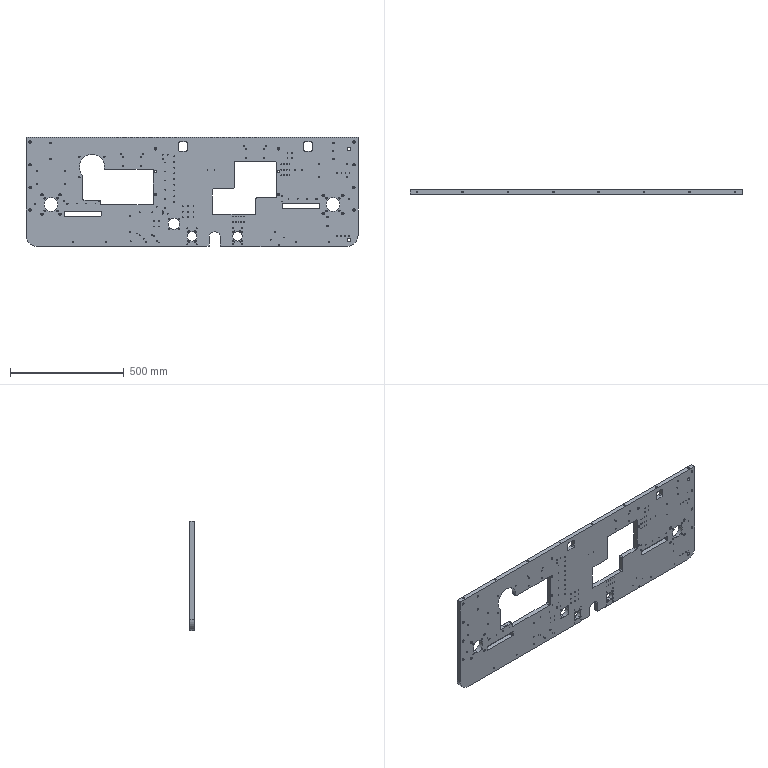Part | STEP file | ND25021-01-JDKM-02-TL | 1 solid | 723 faces | box 1460 x 20 x 480 mm | volume 11435283 mm3 | cylinder 565 | cone 80 | plane 78 | commonest cylinder face diameters 4.2 x160 3.3 x106 5 x70 6.6 x52 11 x52 6.8 x32